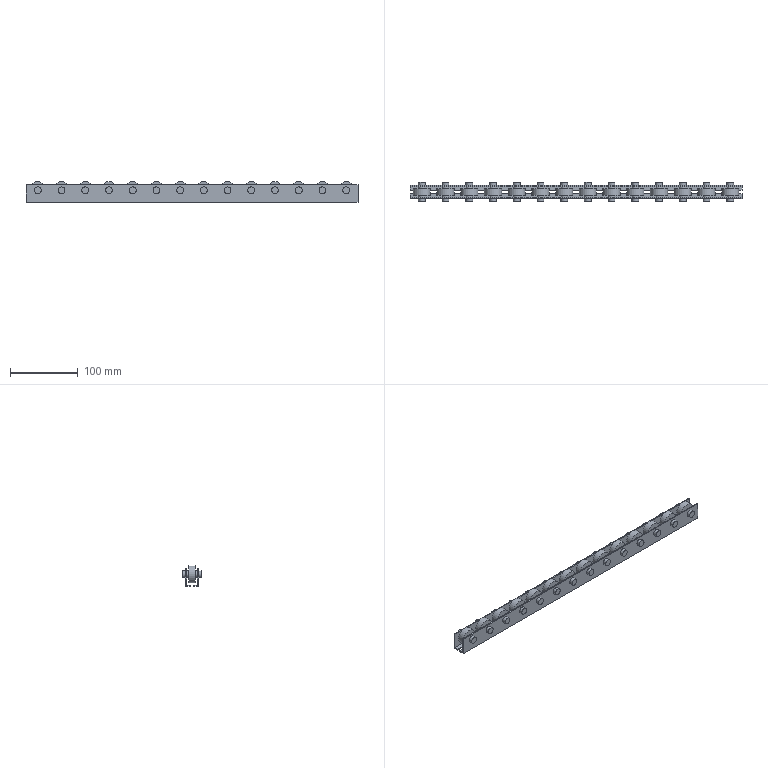Part | NX | features solid 2 | 1 solid | 142 faces | box 490 x 29 x 30.5 mm | volume 131553 mm3 | plane 72 | cylinder 70 | commonest cylinder face diameters 10 x56 25.4 x14